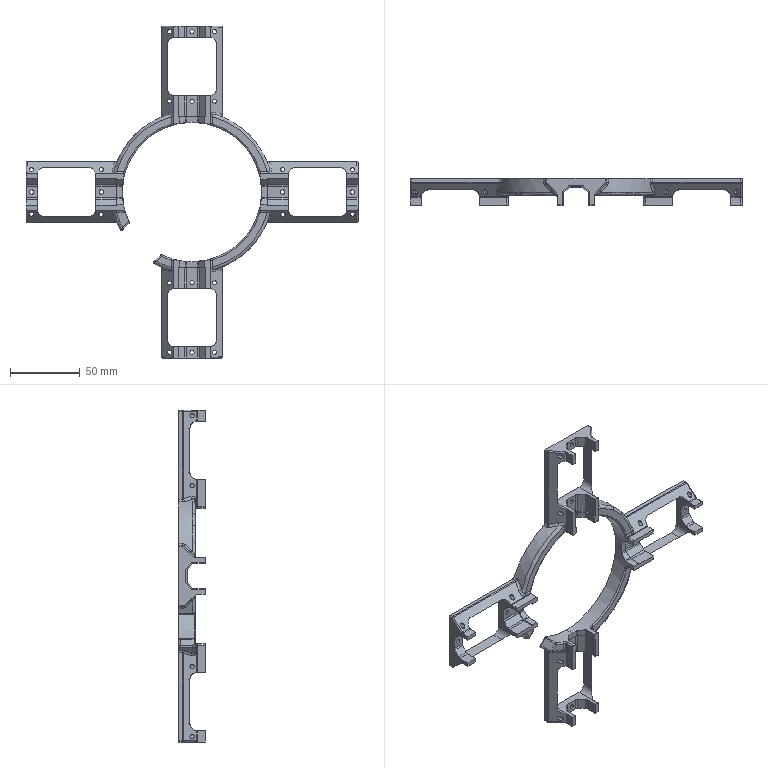Part | SolidWorks | features ICE 9, Fillet 5, MirrorPattern 3, Extrusion 1 | 1 solid | 406 faces | box 238 x 19 x 238 mm | volume 66674 mm3 | cylinder 195 | plane 140 | spline 54 | torus 9 | sphere 8 | commonest cylinder face diameters 2 x75 3 x48 4 x48 10 x16 116 x5 100 x3